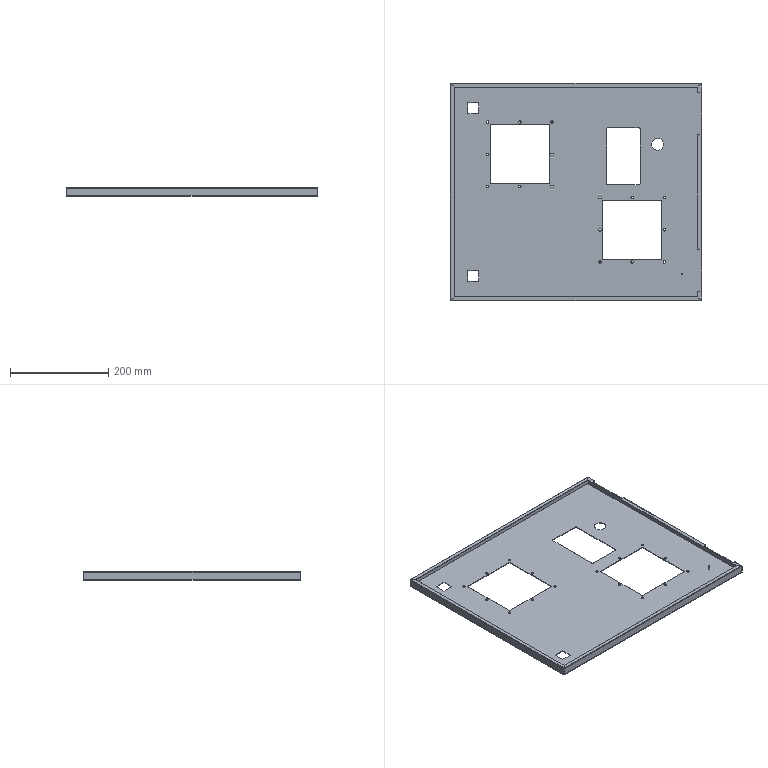Part | STEP file | 1 solid | 171 faces | box 513 x 444 x 17 mm | volume 274646 mm3 | plane 95 | cylinder 64 | spline 12 | commonest cylinder face diameters 5 x32 0.02 x10 2.42 x10 2 x4 4 x4 3 x2